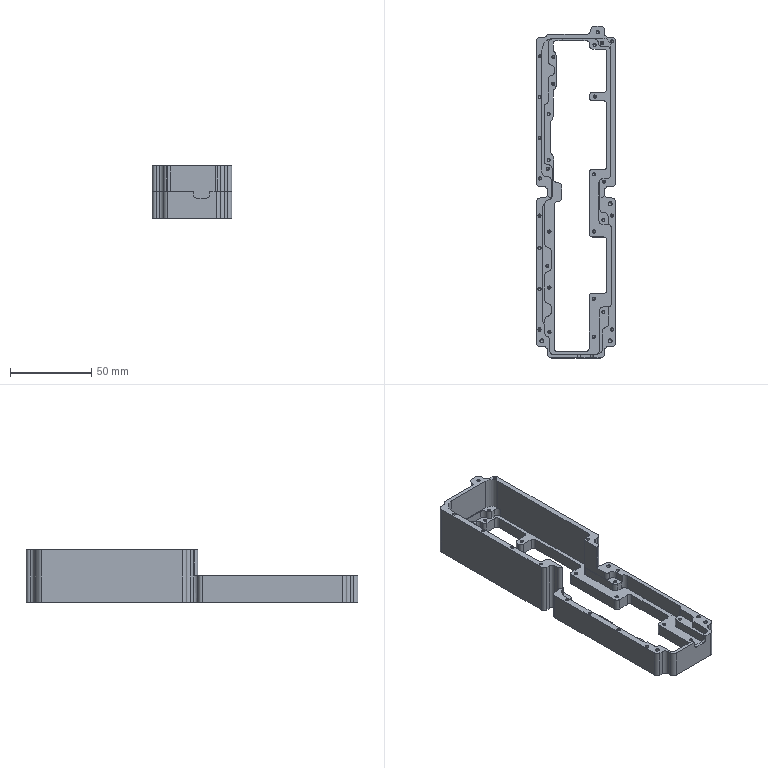Part | STEP file | Final stage amplifier cavity | 1 solid | 344 faces | box 49 x 204 x 32.1 mm | volume 62849 mm3 | cylinder 150 | cone 104 | plane 90 | commonest cylinder face diameters 1.6 x31 4 x28 5 x25 5.2 x18 2.5 x16 4.8 x14